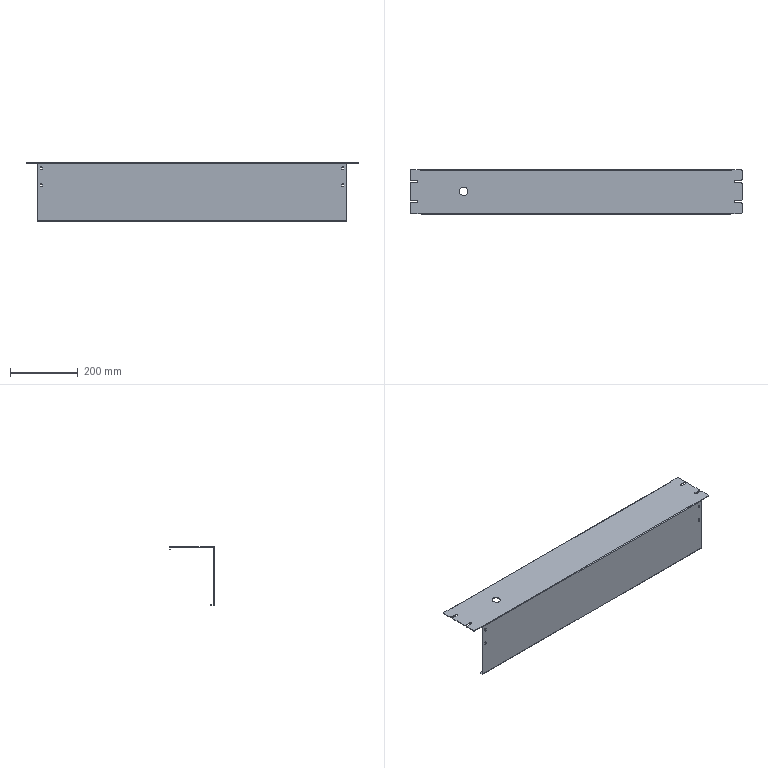Part | STEP file | Rear Sheet Metal Cover Plate | 1 solid | 98 faces | box 980 x 132 x 174.1 mm | volume 597177 mm3 | plane 54 | cylinder 44 | commonest cylinder face diameters 4 x18 4.5 x12 6.5 x6 0.2 x3 4.2 x3 25 x2